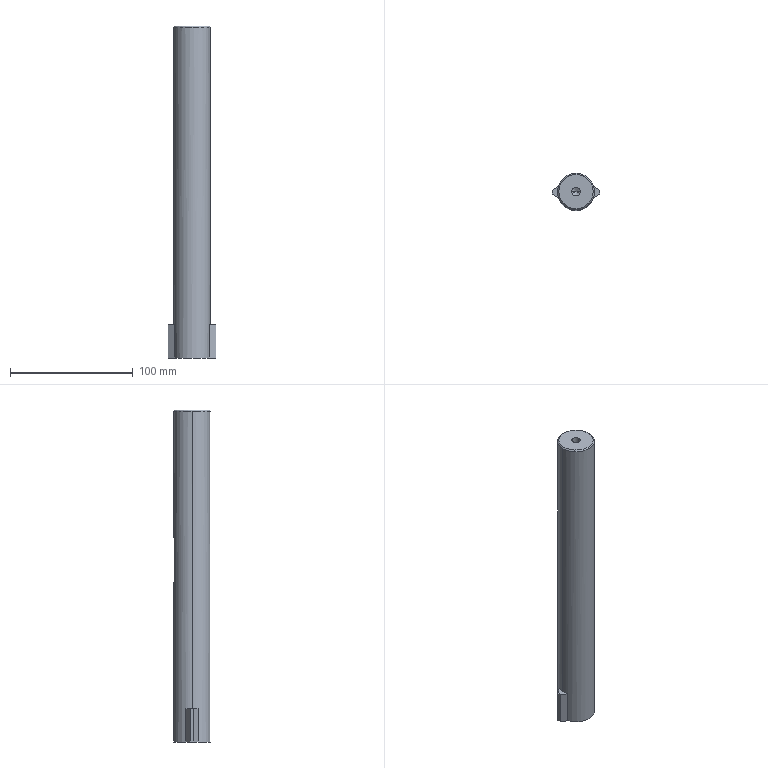Part | STEP file | SHAFT_DIA30_BOTTOM_MOUNTINGV11 | 1 solid | 24 faces | box 39 x 30 x 270 mm | volume 190340 mm3 | plane 13 | cylinder 7 | cone 4 | commonest cylinder face diameters 8 x3 6.8 x2 30 x2